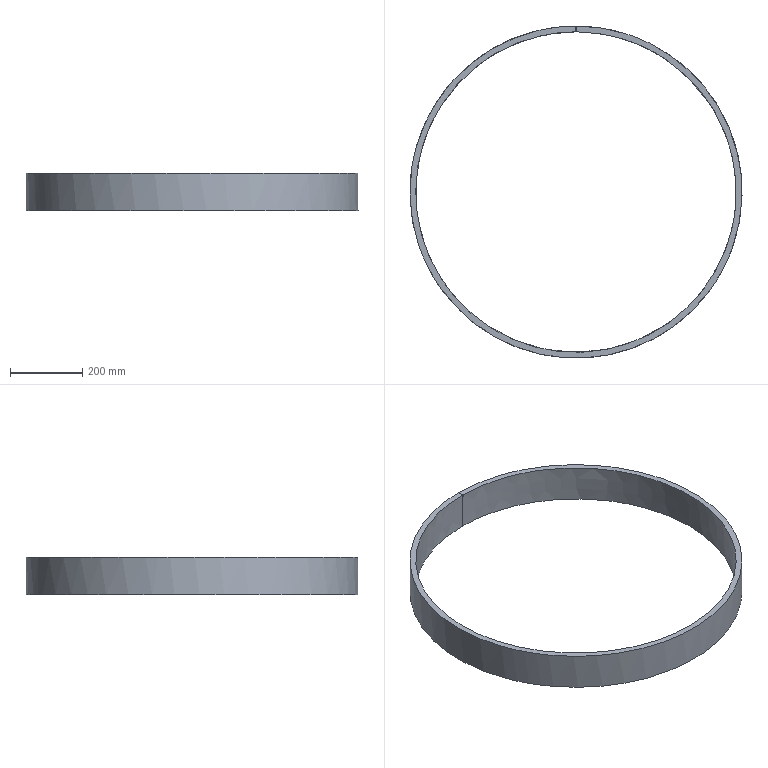Part | SolidWorks | features FlatPattern 1, LoftedBend 1, SheetMetal 1 | 1 solid | 6 faces | box 920 x 920.001 x 105 mm | volume 4770127 mm3 | spline 5 | plane 1